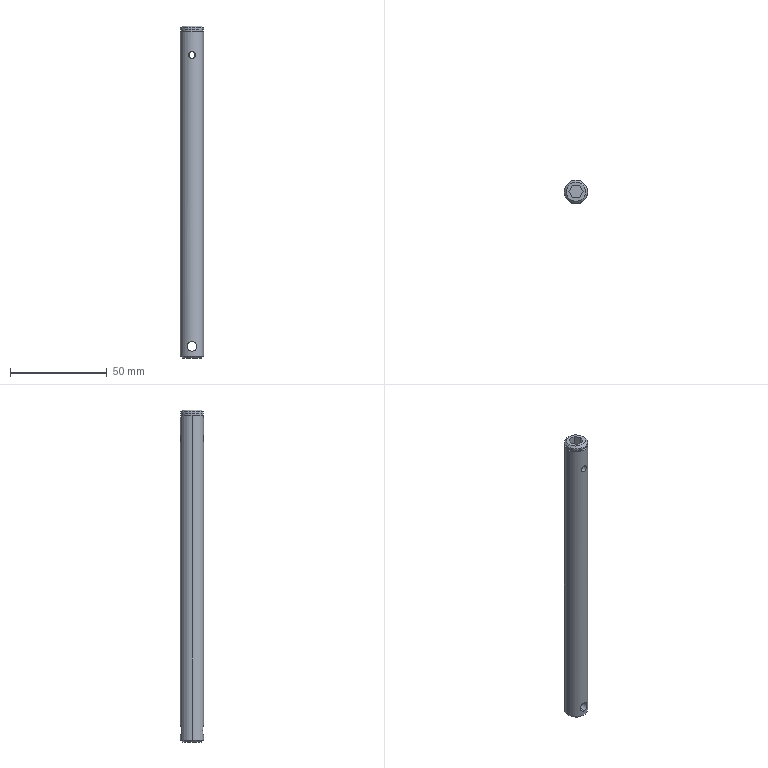Part | STEP file | Rotating rod | 1 solid | 33 faces | box 12 x 12 x 172 mm | volume 18082 mm3 | cylinder 16 | plane 13 | cone 4 | commonest cylinder face diameters 3.2 x4 3.6 x4 12 x4 5 x2 11 x2